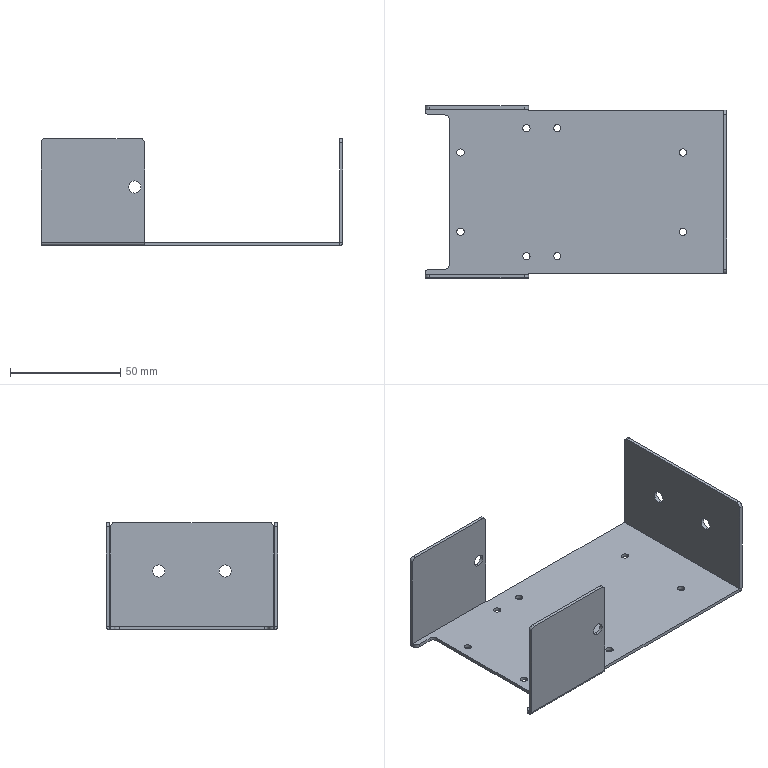Part | STEP file | energy chain clamp plate | 1 solid | 72 faces | box 137 x 78 x 48.5 mm | volume 25843 mm3 | cylinder 40 | plane 32 | commonest cylinder face diameters 3.3 x16 4 x10 5.5 x8 0.02 x3 3.02 x3